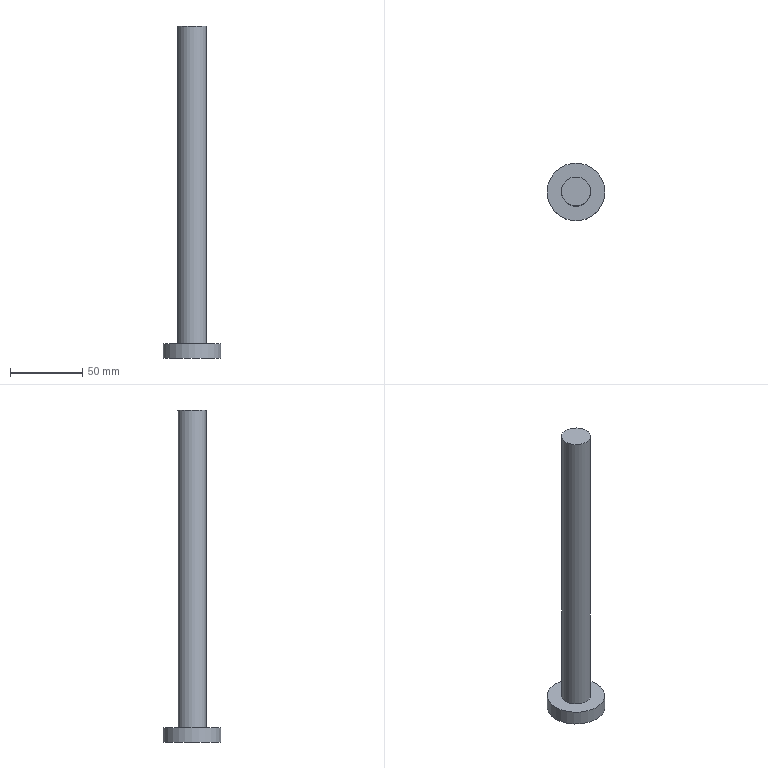Part | NX | features 推移千斤顶约束销 2 | 1 solid | 5 faces | box 40 x 40 x 230 mm | volume 81681 mm3 | plane 3 | cylinder 2 | commonest cylinder face diameters 20 x1 40 x1
STEP:
#1=CARTESIAN_POINT('',(10.,0.,220.));
#2=VERTEX_POINT('',#1);
#3=CARTESIAN_POINT('',(0.,0.,220.));
#4=DIRECTION('',(0.,0.,1.));
#5=DIRECTION('',(1.,0.,0.));
#6=AXIS2_PLACEMENT_3D('',#3,#4,#5);
#7=CIRCLE('',#6,10.);
#8=EDGE_CURVE('',#2,#2,#7,.T.);
#9=ORIENTED_EDGE('',*,*,#8,.F.);
#10=EDGE_LOOP('',(#9));
#11=FACE_BOUND('',#10,.T.);
#12=CARTESIAN_POINT('',(-10.,0.,0.));
#13=VERTEX_POINT('',#12);
#14=CARTESIAN_POINT('',(0.,0.,0.));
#15=DIRECTION('',(0.,0.,-1.));
#16=DIRECTION('',(-1.,0.,0.));
#17=AXIS2_PLACEMENT_3D('',#14,#15,#16);
#18=CIRCLE('',#17,10.);
#19=EDGE_CURVE('',#13,#13,#18,.T.);
#20=ORIENTED_EDGE('',*,*,#19,.F.);
#21=EDGE_LOOP('',(#20));
#22=FACE_BOUND('',#21,.T.);
#23=CARTESIAN_POINT('',(0.,0.,220.));
#24=DIRECTION('',(0.,0.,-1.));
#25=DIRECTION('',(-1.,0.,0.));
#26=AXIS2_PLACEMENT_3D('',#23,#24,#25);
#27=CYLINDRICAL_SURFACE('',#26,10.);
#28=ADVANCED_FACE('',(#11,#22),#27,.T.);
#29=ORIENTED_EDGE('',*,*,#8,.T.);
#30=EDGE_LOOP('',(#29));
#31=FACE_BOUND('',#30,.T.);
#32=CARTESIAN_POINT('',(0.,0.,220.));
#33=DIRECTION('',(0.,0.,1.));
#34=DIRECTION('',(1.,0.,0.));
#35=AXIS2_PLACEMENT_3D('',#32,#33,#34);
#36=PLANE('',#35);
#37=ADVANCED_FACE('',(#31),#36,.T.);
#38=CARTESIAN_POINT('',(-20.,0.,0.));
#39=VERTEX_POINT('',#38);
#40=CARTESIAN_POINT('',(0.,0.,0.));
#41=DIRECTION('',(0.,0.,-1.));
#42=DIRECTION('',(-1.,0.,0.));
#43=AXIS2_PLACEMENT_3D('',#40,#41,#42);
#44=CIRCLE('',#43,20.);
#45=EDGE_CURVE('',#39,#39,#44,.T.);
#46=ORIENTED_EDGE('',*,*,#45,.F.);
#47=EDGE_LOOP('',(#46));
#48=FACE_BOUND('',#47,.T.);
#49=ORIENTED_EDGE('',*,*,#19,.T.);
#50=EDGE_LOOP('',(#49));
#51=FACE_BOUND('',#50,.T.);
#52=CARTESIAN_POINT('',(0.,0.,0.));
#53=DIRECTION('',(0.,0.,-1.));
#54=DIRECTION('',(-1.,0.,0.));
#55=AXIS2_PLACEMENT_3D('',#52,#53,#54);
#56=PLANE('',#55);
#57=ADVANCED_FACE('',(#48,#51),#56,.F.);
#58=CARTESIAN_POINT('',(-20.,0.,-10.));
#59=VERTEX_POINT('',#58);
#60=CARTESIAN_POINT('',(0.,0.,-10.));
#61=DIRECTION('',(0.,0.,-1.));
#62=DIRECTION('',(-1.,0.,0.));
#63=AXIS2_PLACEMENT_3D('',#60,#61,#62);
#64=CIRCLE('',#63,20.);
#65=EDGE_CURVE('',#59,#59,#64,.T.);
#66=ORIENTED_EDGE('',*,*,#65,.F.);
#67=EDGE_LOOP('',(#66));
#68=FACE_BOUND('',#67,.T.);
#69=ORIENTED_EDGE('',*,*,#45,.T.);
#70=EDGE_LOOP('',(#69));
#71=FACE_BOUND('',#70,.T.);
#72=CARTESIAN_POINT('',(0.,0.,-10.));
#73=DIRECTION('',(0.,0.,1.));
#74=DIRECTION('',(1.,0.,0.));
#75=AXIS2_PLACEMENT_3D('',#72,#73,#74);
#76=CYLINDRICAL_SURFACE('',#75,20.);
#77=ADVANCED_FACE('',(#68,#71),#76,.T.);
#78=ORIENTED_EDGE('',*,*,#65,.T.);
#79=EDGE_LOOP('',(#78));
#80=FACE_BOUND('',#79,.T.);
#81=CARTESIAN_POINT('',(0.,0.,-10.));
#82=DIRECTION('',(0.,0.,-1.));
#83=DIRECTION('',(-1.,0.,0.));
#84=AXIS2_PLACEMENT_3D('',#81,#82,#83);
#85=PLANE('',#84);
#86=ADVANCED_FACE('',(#80),#85,.T.);
#87=CLOSED_SHELL('',(#28,#37,#57,#77,#86));
#88=MANIFOLD_SOLID_BREP('',#87);
#89=(LENGTH_UNIT()NAMED_UNIT(*)SI_UNIT(.MILLI.,.METRE.));
#90=UNCERTAINTY_MEASURE_WITH_UNIT(LENGTH_MEASURE(0.00001),#89,'','');
#91=(NAMED_UNIT(*)PLANE_ANGLE_UNIT()SI_UNIT($,.RADIAN.));
#92=(NAMED_UNIT(*)SI_UNIT($,.STERADIAN.)SOLID_ANGLE_UNIT());
#93=(GEOMETRIC_REPRESENTATION_CONTEXT(3)GLOBAL_UNCERTAINTY_ASSIGNED_CONTEXT((#90))GLOBAL_UNIT_ASSIGNED_CONTEXT((#89,#91,#92))REPRESENTATION_CONTEXT('',''));
#94=ADVANCED_BREP_SHAPE_REPRESENTATION('',(#88),#93);